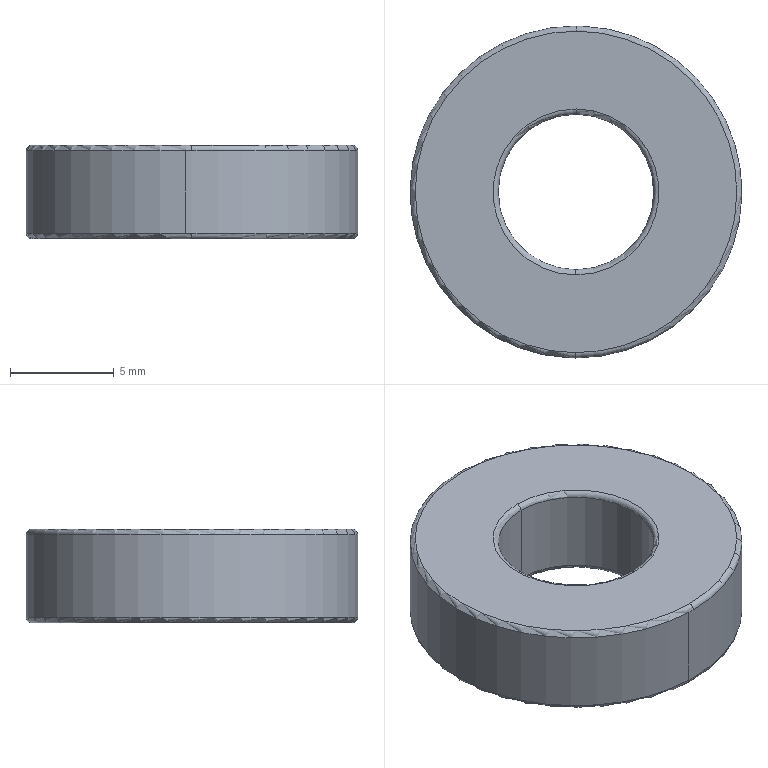Part | STEP file | 2026.6.15-Main Assembly图.sldasm-Part-121 | 1 solid | 14 faces | box 16 x 16 x 4.5 mm | volume 703.994 mm3 | torus 8 | cylinder 4 | plane 2 | commonest cylinder face diameters 7.5 x2 16 x2
STEP:
#1=CARTESIAN_POINT('',(-1571.259,1416.256,3701.821));
#2=VERTEX_POINT('',#1);
#3=CARTESIAN_POINT('',(-1570.942,1432.25,3701.821));
#4=VERTEX_POINT('',#3);
#5=CARTESIAN_POINT('',(-1571.253,1424.256,3701.821));
#6=DIRECTION('',(0.,0.,1.));
#7=DIRECTION('',(0.0007664,1.,0.));
#8=AXIS2_PLACEMENT_3D('',#5,#6,#7);
#9=CIRCLE('',#8,8.);
#10=EDGE_CURVE('',#2,#4,#9,.T.);
#11=ORIENTED_EDGE('',*,*,#10,.F.);
#12=CARTESIAN_POINT('',(-1571.259,1416.506,3701.571));
#13=VERTEX_POINT('',#12);
#14=CARTESIAN_POINT('',(-1571.259,1416.506,3701.821));
#15=DIRECTION('',(1.,-0.0007664,0.));
#16=DIRECTION('',(0.0007664,1.,0.));
#17=AXIS2_PLACEMENT_3D('',#14,#15,#16);
#18=CIRCLE('',#17,0.25);
#19=EDGE_CURVE('',#2,#13,#18,.T.);
#20=ORIENTED_EDGE('',*,*,#19,.T.);
#21=CARTESIAN_POINT('',(-1571.247,1432.006,3701.571));
#22=VERTEX_POINT('',#21);
#23=CARTESIAN_POINT('',(-1571.253,1424.256,3701.571));
#24=DIRECTION('',(0.,0.,-1.));
#25=DIRECTION('',(0.0007664,1.,0.));
#26=AXIS2_PLACEMENT_3D('',#23,#24,#25);
#27=CIRCLE('',#26,7.75);
#28=EDGE_CURVE('',#22,#13,#27,.T.);
#29=ORIENTED_EDGE('',*,*,#28,.F.);
#30=CARTESIAN_POINT('',(-1571.247,1432.256,3701.821));
#31=VERTEX_POINT('',#30);
#32=CARTESIAN_POINT('',(-1571.247,1432.006,3701.821));
#33=DIRECTION('',(-1.,0.0007664,0.));
#34=DIRECTION('',(-0.0007664,-1.,0.));
#35=AXIS2_PLACEMENT_3D('',#32,#33,#34);
#36=CIRCLE('',#35,0.25);
#37=EDGE_CURVE('',#31,#22,#36,.T.);
#38=ORIENTED_EDGE('',*,*,#37,.F.);
#39=CARTESIAN_POINT('',(-1571.253,1424.256,3701.821));
#40=DIRECTION('',(0.,0.,1.));
#41=DIRECTION('',(0.0007664,1.,0.));
#42=AXIS2_PLACEMENT_3D('',#39,#40,#41);
#43=CIRCLE('',#42,8.);
#44=EDGE_CURVE('',#4,#31,#43,.T.);
#45=ORIENTED_EDGE('',*,*,#44,.F.);
#46=EDGE_LOOP('',(#11,#20,#29,#38,#45));
#47=FACE_OUTER_BOUND('',#46,.T.);
#48=CARTESIAN_POINT('',(-1571.253,1424.256,3701.821));
#49=DIRECTION('',(0.,0.,-1.));
#50=DIRECTION('',(0.0007664,1.,0.));
#51=AXIS2_PLACEMENT_3D('',#48,#49,#50);
#52=TOROIDAL_SURFACE('',#51,7.75,0.25);
#53=ADVANCED_FACE('',(#47),#52,.T.);
#54=CARTESIAN_POINT('',(-1571.247,1432.256,3705.821));
#55=VERTEX_POINT('',#54);
#56=CARTESIAN_POINT('',(-1570.942,1432.25,3705.821));
#57=VERTEX_POINT('',#56);
#58=CARTESIAN_POINT('',(-1571.253,1424.256,3705.821));
#59=DIRECTION('',(0.,0.,-1.));
#60=DIRECTION('',(-0.0007664,-1.,0.));
#61=AXIS2_PLACEMENT_3D('',#58,#59,#60);
#62=CIRCLE('',#61,8.);
#63=EDGE_CURVE('',#55,#57,#62,.T.);
#64=ORIENTED_EDGE('',*,*,#63,.F.);
#65=CARTESIAN_POINT('',(-1571.247,1432.006,3706.071));
#66=VERTEX_POINT('',#65);
#67=CARTESIAN_POINT('',(-1571.247,1432.006,3705.821));
#68=DIRECTION('',(1.,-0.0007664,0.));
#69=DIRECTION('',(0.0007664,1.,0.));
#70=AXIS2_PLACEMENT_3D('',#67,#68,#69);
#71=CIRCLE('',#70,0.25);
#72=EDGE_CURVE('',#55,#66,#71,.T.);
#73=ORIENTED_EDGE('',*,*,#72,.T.);
#74=CARTESIAN_POINT('',(-1571.259,1416.506,3706.071));
#75=VERTEX_POINT('',#74);
#76=CARTESIAN_POINT('',(-1571.253,1424.256,3706.071));
#77=DIRECTION('',(0.,0.,1.));
#78=DIRECTION('',(-0.0007664,-1.,0.));
#79=AXIS2_PLACEMENT_3D('',#76,#77,#78);
#80=CIRCLE('',#79,7.75);
#81=EDGE_CURVE('',#75,#66,#80,.T.);
#82=ORIENTED_EDGE('',*,*,#81,.F.);
#83=CARTESIAN_POINT('',(-1571.259,1416.256,3705.821));
#84=VERTEX_POINT('',#83);
#85=CARTESIAN_POINT('',(-1571.259,1416.506,3705.821));
#86=DIRECTION('',(-1.,0.0007664,0.));
#87=DIRECTION('',(-0.0007664,-1.,0.));
#88=AXIS2_PLACEMENT_3D('',#85,#86,#87);
#89=CIRCLE('',#88,0.25);
#90=EDGE_CURVE('',#84,#75,#89,.T.);
#91=ORIENTED_EDGE('',*,*,#90,.F.);
#92=CARTESIAN_POINT('',(-1571.253,1424.256,3705.821));
#93=DIRECTION('',(0.,0.,-1.));
#94=DIRECTION('',(-0.0007664,-1.,0.));
#95=AXIS2_PLACEMENT_3D('',#92,#93,#94);
#96=CIRCLE('',#95,8.);
#97=EDGE_CURVE('',#57,#84,#96,.T.);
#98=ORIENTED_EDGE('',*,*,#97,.F.);
#99=EDGE_LOOP('',(#64,#73,#82,#91,#98));
#100=FACE_OUTER_BOUND('',#99,.T.);
#101=CARTESIAN_POINT('',(-1571.253,1424.256,3705.821));
#102=DIRECTION('',(0.,0.,1.));
#103=DIRECTION('',(-0.0007664,-1.,0.));
#104=AXIS2_PLACEMENT_3D('',#101,#102,#103);
#105=TOROIDAL_SURFACE('',#104,7.75,0.25);
#106=ADVANCED_FACE('',(#100),#105,.T.);
#107=CARTESIAN_POINT('',(-1571.25,1428.256,3706.071));
#108=VERTEX_POINT('',#107);
#109=CARTESIAN_POINT('',(-1571.256,1420.256,3706.071));
#110=VERTEX_POINT('',#109);
#111=CARTESIAN_POINT('',(-1571.253,1424.256,3706.071));
#112=DIRECTION('',(0.,0.,-1.));
#113=DIRECTION('',(-0.0007664,-1.,0.));
#114=AXIS2_PLACEMENT_3D('',#111,#112,#113);
#115=CIRCLE('',#114,4.);
#116=EDGE_CURVE('',#108,#110,#115,.T.);
#117=ORIENTED_EDGE('',*,*,#116,.F.);
#118=CARTESIAN_POINT('',(-1571.25,1428.006,3705.821));
#119=VERTEX_POINT('',#118);
#120=CARTESIAN_POINT('',(-1571.25,1428.256,3705.821));
#121=DIRECTION('',(1.,-0.0007664,0.));
#122=DIRECTION('',(0.0007664,1.,0.));
#123=AXIS2_PLACEMENT_3D('',#120,#121,#122);
#124=CIRCLE('',#123,0.25);
#125=EDGE_CURVE('',#108,#119,#124,.T.);
#126=ORIENTED_EDGE('',*,*,#125,.T.);
#127=CARTESIAN_POINT('',(-1571.256,1420.506,3705.821));
#128=VERTEX_POINT('',#127);
#129=CARTESIAN_POINT('',(-1571.253,1424.256,3705.821));
#130=DIRECTION('',(0.,0.,1.));
#131=DIRECTION('',(-0.0007664,-1.,0.));
#132=AXIS2_PLACEMENT_3D('',#129,#130,#131);
#133=CIRCLE('',#132,3.75);
#134=EDGE_CURVE('',#128,#119,#133,.T.);
#135=ORIENTED_EDGE('',*,*,#134,.F.);
#136=CARTESIAN_POINT('',(-1571.256,1420.256,3705.821));
#137=DIRECTION('',(-1.,0.0007664,0.));
#138=DIRECTION('',(-0.0007664,-1.,0.));
#139=AXIS2_PLACEMENT_3D('',#136,#137,#138);
#140=CIRCLE('',#139,0.25);
#141=EDGE_CURVE('',#110,#128,#140,.T.);
#142=ORIENTED_EDGE('',*,*,#141,.F.);
#143=EDGE_LOOP('',(#117,#126,#135,#142));
#144=FACE_OUTER_BOUND('',#143,.T.);
#145=CARTESIAN_POINT('',(-1571.253,1424.256,3705.821));
#146=DIRECTION('',(0.,0.,1.));
#147=DIRECTION('',(-0.0007664,-1.,0.));
#148=AXIS2_PLACEMENT_3D('',#145,#146,#147);
#149=TOROIDAL_SURFACE('',#148,4.,0.25);
#150=ADVANCED_FACE('',(#144),#149,.T.);
#151=CARTESIAN_POINT('',(-1571.256,1420.256,3701.571));
#152=VERTEX_POINT('',#151);
#153=CARTESIAN_POINT('',(-1571.25,1428.256,3701.571));
#154=VERTEX_POINT('',#153);
#155=CARTESIAN_POINT('',(-1571.253,1424.256,3701.571));
#156=DIRECTION('',(0.,0.,1.));
#157=DIRECTION('',(0.0007664,1.,0.));
#158=AXIS2_PLACEMENT_3D('',#155,#156,#157);
#159=CIRCLE('',#158,4.);
#160=EDGE_CURVE('',#152,#154,#159,.T.);
#161=ORIENTED_EDGE('',*,*,#160,.F.);
#162=CARTESIAN_POINT('',(-1571.256,1420.506,3701.821));
#163=VERTEX_POINT('',#162);
#164=CARTESIAN_POINT('',(-1571.256,1420.256,3701.821));
#165=DIRECTION('',(1.,-0.0007664,0.));
#166=DIRECTION('',(0.0007664,1.,0.));
#167=AXIS2_PLACEMENT_3D('',#164,#165,#166);
#168=CIRCLE('',#167,0.25);
#169=EDGE_CURVE('',#152,#163,#168,.T.);
#170=ORIENTED_EDGE('',*,*,#169,.T.);
#171=CARTESIAN_POINT('',(-1571.25,1428.006,3701.821));
#172=VERTEX_POINT('',#171);
#173=CARTESIAN_POINT('',(-1571.253,1424.256,3701.821));
#174=DIRECTION('',(0.,0.,-1.));
#175=DIRECTION('',(0.0007664,1.,0.));
#176=AXIS2_PLACEMENT_3D('',#173,#174,#175);
#177=CIRCLE('',#176,3.75);
#178=EDGE_CURVE('',#172,#163,#177,.T.);
#179=ORIENTED_EDGE('',*,*,#178,.F.);
#180=CARTESIAN_POINT('',(-1571.25,1428.256,3701.821));
#181=DIRECTION('',(-1.,0.0007664,0.));
#182=DIRECTION('',(-0.0007664,-1.,0.));
#183=AXIS2_PLACEMENT_3D('',#180,#181,#182);
#184=CIRCLE('',#183,0.25);
#185=EDGE_CURVE('',#154,#172,#184,.T.);
#186=ORIENTED_EDGE('',*,*,#185,.F.);
#187=EDGE_LOOP('',(#161,#170,#179,#186));
#188=FACE_OUTER_BOUND('',#187,.T.);
#189=CARTESIAN_POINT('',(-1571.253,1424.256,3701.821));
#190=DIRECTION('',(0.,0.,-1.));
#191=DIRECTION('',(0.0007664,1.,0.));
#192=AXIS2_PLACEMENT_3D('',#189,#190,#191);
#193=TOROIDAL_SURFACE('',#192,4.,0.25);
#194=ADVANCED_FACE('',(#188),#193,.T.);
#195=CARTESIAN_POINT('',(-1571.253,1424.256,3701.821));
#196=DIRECTION('',(0.,0.,-1.));
#197=DIRECTION('',(0.0007664,1.,0.));
#198=AXIS2_PLACEMENT_3D('',#195,#196,#197);
#199=CIRCLE('',#198,3.75);
#200=EDGE_CURVE('',#163,#172,#199,.T.);
#201=ORIENTED_EDGE('',*,*,#200,.T.);
#202=CARTESIAN_POINT('',(-1571.25,1428.006,3701.571));
#203=DIRECTION('',(0.,0.,1.));
#204=VECTOR('',#203,1000.);
#205=LINE('',#202,#204);
#206=EDGE_CURVE('',#172,#119,#205,.T.);
#207=ORIENTED_EDGE('',*,*,#206,.T.);
#208=CARTESIAN_POINT('',(-1571.253,1424.256,3705.821));
#209=DIRECTION('',(0.,0.,1.));
#210=DIRECTION('',(-0.0007664,-1.,0.));
#211=AXIS2_PLACEMENT_3D('',#208,#209,#210);
#212=CIRCLE('',#211,3.75);
#213=EDGE_CURVE('',#119,#128,#212,.T.);
#214=ORIENTED_EDGE('',*,*,#213,.T.);
#215=CARTESIAN_POINT('',(-1571.256,1420.506,3701.571));
#216=DIRECTION('',(0.,0.,1.));
#217=VECTOR('',#216,1000.);
#218=LINE('',#215,#217);
#219=EDGE_CURVE('',#163,#128,#218,.T.);
#220=ORIENTED_EDGE('',*,*,#219,.F.);
#221=EDGE_LOOP('',(#201,#207,#214,#220));
#222=FACE_OUTER_BOUND('',#221,.T.);
#223=CARTESIAN_POINT('',(-1571.253,1424.256,3701.571));
#224=DIRECTION('',(0.,0.,1.));
#225=DIRECTION('',(-0.0007664,-1.,0.));
#226=AXIS2_PLACEMENT_3D('',#223,#224,#225);
#227=CYLINDRICAL_SURFACE('',#226,3.75);
#228=ADVANCED_FACE('',(#222),#227,.F.);
#229=ORIENTED_EDGE('',*,*,#97,.T.);
#230=CARTESIAN_POINT('',(-1571.565,1416.262,3705.821));
#231=VERTEX_POINT('',#230);
#232=CARTESIAN_POINT('',(-1571.253,1424.256,3705.821));
#233=DIRECTION('',(0.,0.,-1.));
#234=DIRECTION('',(-0.0007664,-1.,0.));
#235=AXIS2_PLACEMENT_3D('',#232,#233,#234);
#236=CIRCLE('',#235,8.);
#237=EDGE_CURVE('',#84,#231,#236,.T.);
#238=ORIENTED_EDGE('',*,*,#237,.T.);
#239=CARTESIAN_POINT('',(-1571.565,1416.262,3701.821));
#240=VERTEX_POINT('',#239);
#241=CARTESIAN_POINT('',(-1571.565,1416.262,3706.071));
#242=DIRECTION('',(0.,0.,-1.));
#243=VECTOR('',#242,1000.);
#244=LINE('',#241,#243);
#245=EDGE_CURVE('',#231,#240,#244,.T.);
#246=ORIENTED_EDGE('',*,*,#245,.T.);
#247=CARTESIAN_POINT('',(-1571.253,1424.256,3701.821));
#248=DIRECTION('',(0.,0.,1.));
#249=DIRECTION('',(0.0007664,1.,0.));
#250=AXIS2_PLACEMENT_3D('',#247,#248,#249);
#251=CIRCLE('',#250,8.);
#252=EDGE_CURVE('',#240,#2,#251,.T.);
#253=ORIENTED_EDGE('',*,*,#252,.T.);
#254=ORIENTED_EDGE('',*,*,#10,.T.);
#255=CARTESIAN_POINT('',(-1570.942,1432.25,3706.071));
#256=DIRECTION('',(0.,0.,-1.));
#257=VECTOR('',#256,1000.);
#258=LINE('',#255,#257);
#259=EDGE_CURVE('',#57,#4,#258,.T.);
#260=ORIENTED_EDGE('',*,*,#259,.F.);
#261=EDGE_LOOP('',(#229,#238,#246,#253,#254,#260));
#262=FACE_OUTER_BOUND('',#261,.T.);
#263=CARTESIAN_POINT('',(-1571.253,1424.256,3706.071));
#264=DIRECTION('',(0.,0.,-1.));
#265=DIRECTION('',(0.03892,0.9992,0.));
#266=AXIS2_PLACEMENT_3D('',#263,#264,#265);
#267=CYLINDRICAL_SURFACE('',#266,8.);
#268=ADVANCED_FACE('',(#262),#267,.T.);
#269=CARTESIAN_POINT('',(-1571.253,1424.256,3701.571));
#270=DIRECTION('',(0.,0.,1.));
#271=DIRECTION('',(0.0007664,1.,0.));
#272=AXIS2_PLACEMENT_3D('',#269,#270,#271);
#273=CIRCLE('',#272,4.);
#274=EDGE_CURVE('',#154,#152,#273,.T.);
#275=ORIENTED_EDGE('',*,*,#274,.T.);
#276=ORIENTED_EDGE('',*,*,#160,.T.);
#277=EDGE_LOOP('',(#275,#276));
#278=FACE_BOUND('',#277,.T.);
#279=ORIENTED_EDGE('',*,*,#28,.T.);
#280=CARTESIAN_POINT('',(-1571.253,1424.256,3701.571));
#281=DIRECTION('',(0.,0.,-1.));
#282=DIRECTION('',(0.0007664,1.,0.));
#283=AXIS2_PLACEMENT_3D('',#280,#281,#282);
#284=CIRCLE('',#283,7.75);
#285=EDGE_CURVE('',#13,#22,#284,.T.);
#286=ORIENTED_EDGE('',*,*,#285,.T.);
#287=EDGE_LOOP('',(#279,#286));
#288=FACE_OUTER_BOUND('',#287,.T.);
#289=CARTESIAN_POINT('',(-1571.253,1424.256,3701.571));
#290=DIRECTION('',(0.,0.,-1.));
#291=DIRECTION('',(0.0007664,1.,0.));
#292=AXIS2_PLACEMENT_3D('',#289,#290,#291);
#293=PLANE('',#292);
#294=ADVANCED_FACE('',(#278,#288),#293,.T.);
#295=CARTESIAN_POINT('',(-1571.253,1424.256,3706.071));
#296=DIRECTION('',(0.,0.,-1.));
#297=DIRECTION('',(-0.0007664,-1.,0.));
#298=AXIS2_PLACEMENT_3D('',#295,#296,#297);
#299=CIRCLE('',#298,4.);
#300=EDGE_CURVE('',#110,#108,#299,.T.);
#301=ORIENTED_EDGE('',*,*,#300,.T.);
#302=ORIENTED_EDGE('',*,*,#116,.T.);
#303=EDGE_LOOP('',(#301,#302));
#304=FACE_BOUND('',#303,.T.);
#305=ORIENTED_EDGE('',*,*,#81,.T.);
#306=CARTESIAN_POINT('',(-1571.253,1424.256,3706.071));
#307=DIRECTION('',(0.,0.,1.));
#308=DIRECTION('',(-0.0007664,-1.,0.));
#309=AXIS2_PLACEMENT_3D('',#306,#307,#308);
#310=CIRCLE('',#309,7.75);
#311=EDGE_CURVE('',#66,#75,#310,.T.);
#312=ORIENTED_EDGE('',*,*,#311,.T.);
#313=EDGE_LOOP('',(#305,#312));
#314=FACE_OUTER_BOUND('',#313,.T.);
#315=CARTESIAN_POINT('',(-1571.253,1424.256,3706.071));
#316=DIRECTION('',(0.,0.,1.));
#317=DIRECTION('',(-0.0007664,-1.,0.));
#318=AXIS2_PLACEMENT_3D('',#315,#316,#317);
#319=PLANE('',#318);
#320=ADVANCED_FACE('',(#304,#314),#319,.T.);
#321=ORIENTED_EDGE('',*,*,#245,.F.);
#322=CARTESIAN_POINT('',(-1571.253,1424.256,3705.821));
#323=DIRECTION('',(0.,0.,-1.));
#324=DIRECTION('',(-0.0007664,-1.,0.));
#325=AXIS2_PLACEMENT_3D('',#322,#323,#324);
#326=CIRCLE('',#325,8.);
#327=EDGE_CURVE('',#231,#55,#326,.T.);
#328=ORIENTED_EDGE('',*,*,#327,.T.);
#329=ORIENTED_EDGE('',*,*,#63,.T.);
#330=ORIENTED_EDGE('',*,*,#259,.T.);
#331=ORIENTED_EDGE('',*,*,#44,.T.);
#332=CARTESIAN_POINT('',(-1571.253,1424.256,3701.821));
#333=DIRECTION('',(0.,0.,1.));
#334=DIRECTION('',(0.0007664,1.,0.));
#335=AXIS2_PLACEMENT_3D('',#332,#333,#334);
#336=CIRCLE('',#335,8.);
#337=EDGE_CURVE('',#31,#240,#336,.T.);
#338=ORIENTED_EDGE('',*,*,#337,.T.);
#339=EDGE_LOOP('',(#321,#328,#329,#330,#331,#338));
#340=FACE_OUTER_BOUND('',#339,.T.);
#341=CARTESIAN_POINT('',(-1571.253,1424.256,3706.071));
#342=DIRECTION('',(0.,0.,-1.));
#343=DIRECTION('',(0.03892,0.9992,0.));
#344=AXIS2_PLACEMENT_3D('',#341,#342,#343);
#345=CYLINDRICAL_SURFACE('',#344,8.);
#346=ADVANCED_FACE('',(#340),#345,.T.);
#347=ORIENTED_EDGE('',*,*,#206,.F.);
#348=ORIENTED_EDGE('',*,*,#178,.T.);
#349=ORIENTED_EDGE('',*,*,#219,.T.);
#350=ORIENTED_EDGE('',*,*,#134,.T.);
#351=EDGE_LOOP('',(#347,#348,#349,#350));
#352=FACE_OUTER_BOUND('',#351,.T.);
#353=CARTESIAN_POINT('',(-1571.253,1424.256,3701.571));
#354=DIRECTION('',(0.,0.,1.));
#355=DIRECTION('',(-0.0007664,-1.,0.));
#356=AXIS2_PLACEMENT_3D('',#353,#354,#355);
#357=CYLINDRICAL_SURFACE('',#356,3.75);
#358=ADVANCED_FACE('',(#352),#357,.F.);
#359=ORIENTED_EDGE('',*,*,#169,.F.);
#360=ORIENTED_EDGE('',*,*,#274,.F.);
#361=ORIENTED_EDGE('',*,*,#185,.T.);
#362=ORIENTED_EDGE('',*,*,#200,.F.);
#363=EDGE_LOOP('',(#359,#360,#361,#362));
#364=FACE_OUTER_BOUND('',#363,.T.);
#365=CARTESIAN_POINT('',(-1571.253,1424.256,3701.821));
#366=DIRECTION('',(0.,0.,-1.));
#367=DIRECTION('',(0.0007664,1.,0.));
#368=AXIS2_PLACEMENT_3D('',#365,#366,#367);
#369=TOROIDAL_SURFACE('',#368,4.,0.25);
#370=ADVANCED_FACE('',(#364),#369,.T.);
#371=ORIENTED_EDGE('',*,*,#125,.F.);
#372=ORIENTED_EDGE('',*,*,#300,.F.);
#373=ORIENTED_EDGE('',*,*,#141,.T.);
#374=ORIENTED_EDGE('',*,*,#213,.F.);
#375=EDGE_LOOP('',(#371,#372,#373,#374));
#376=FACE_OUTER_BOUND('',#375,.T.);
#377=CARTESIAN_POINT('',(-1571.253,1424.256,3705.821));
#378=DIRECTION('',(0.,0.,1.));
#379=DIRECTION('',(-0.0007664,-1.,0.));
#380=AXIS2_PLACEMENT_3D('',#377,#378,#379);
#381=TOROIDAL_SURFACE('',#380,4.,0.25);
#382=ADVANCED_FACE('',(#376),#381,.T.);
#383=ORIENTED_EDGE('',*,*,#72,.F.);
#384=ORIENTED_EDGE('',*,*,#327,.F.);
#385=ORIENTED_EDGE('',*,*,#237,.F.);
#386=ORIENTED_EDGE('',*,*,#90,.T.);
#387=ORIENTED_EDGE('',*,*,#311,.F.);
#388=EDGE_LOOP('',(#383,#384,#385,#386,#387));
#389=FACE_OUTER_BOUND('',#388,.T.);
#390=CARTESIAN_POINT('',(-1571.253,1424.256,3705.821));
#391=DIRECTION('',(0.,0.,1.));
#392=DIRECTION('',(-0.0007664,-1.,0.));
#393=AXIS2_PLACEMENT_3D('',#390,#391,#392);
#394=TOROIDAL_SURFACE('',#393,7.75,0.25);
#395=ADVANCED_FACE('',(#389),#394,.T.);
#396=ORIENTED_EDGE('',*,*,#19,.F.);
#397=ORIENTED_EDGE('',*,*,#252,.F.);
#398=ORIENTED_EDGE('',*,*,#337,.F.);
#399=ORIENTED_EDGE('',*,*,#37,.T.);
#400=ORIENTED_EDGE('',*,*,#285,.F.);
#401=EDGE_LOOP('',(#396,#397,#398,#399,#400));
#402=FACE_OUTER_BOUND('',#401,.T.);
#403=CARTESIAN_POINT('',(-1571.253,1424.256,3701.821));
#404=DIRECTION('',(0.,0.,-1.));
#405=DIRECTION('',(0.0007664,1.,0.));
#406=AXIS2_PLACEMENT_3D('',#403,#404,#405);
#407=TOROIDAL_SURFACE('',#406,7.75,0.25);
#408=ADVANCED_FACE('',(#402),#407,.T.);
#409=CLOSED_SHELL('',(#53,#106,#150,#194,#228,#268,#294,#320,#346,#358,#370,#382,#395,#408));
#410=MANIFOLD_SOLID_BREP('',#409);
#411=CARTESIAN_POINT('',(0.,0.,0.));
#412=DIRECTION('',(0.,0.,1.));
#413=DIRECTION('',(1.,0.,0.));
#414=AXIS2_PLACEMENT_3D('',#411,#412,#413);
#415=(LENGTH_UNIT()NAMED_UNIT(*)SI_UNIT(.MILLI.,.METRE.));
#416=UNCERTAINTY_MEASURE_WITH_UNIT(LENGTH_MEASURE(0.00001),#415,'','');
#417=(NAMED_UNIT(*)PLANE_ANGLE_UNIT()SI_UNIT($,.RADIAN.));
#418=(NAMED_UNIT(*)SI_UNIT($,.STERADIAN.)SOLID_ANGLE_UNIT());
#419=(GEOMETRIC_REPRESENTATION_CONTEXT(3)GLOBAL_UNCERTAINTY_ASSIGNED_CONTEXT((#416))GLOBAL_UNIT_ASSIGNED_CONTEXT((#415,#417,#418))REPRESENTATION_CONTEXT('',''));
#420=ADVANCED_BREP_SHAPE_REPRESENTATION('',(#410,#414),#419);